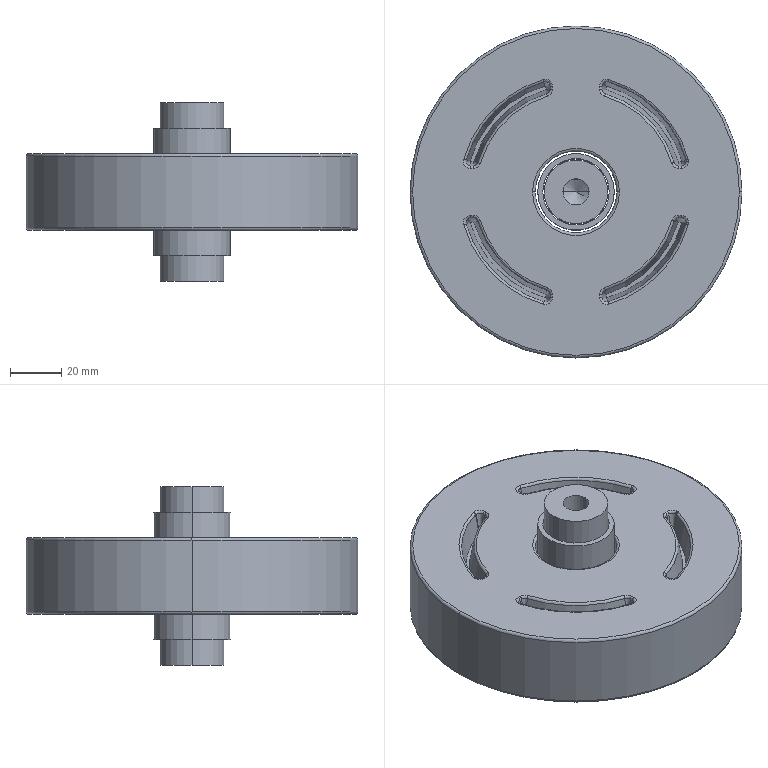Part | SolidWorks | 4 solids | 207 faces | box 130 x 130 x 70 mm | volume 366307 mm3 | torus 60 | cone 60 | cylinder 48 | plane 39 | commonest cylinder face diameters 2 x16 3 x6 10.2 x4 26 x4 30 x4 52 x4